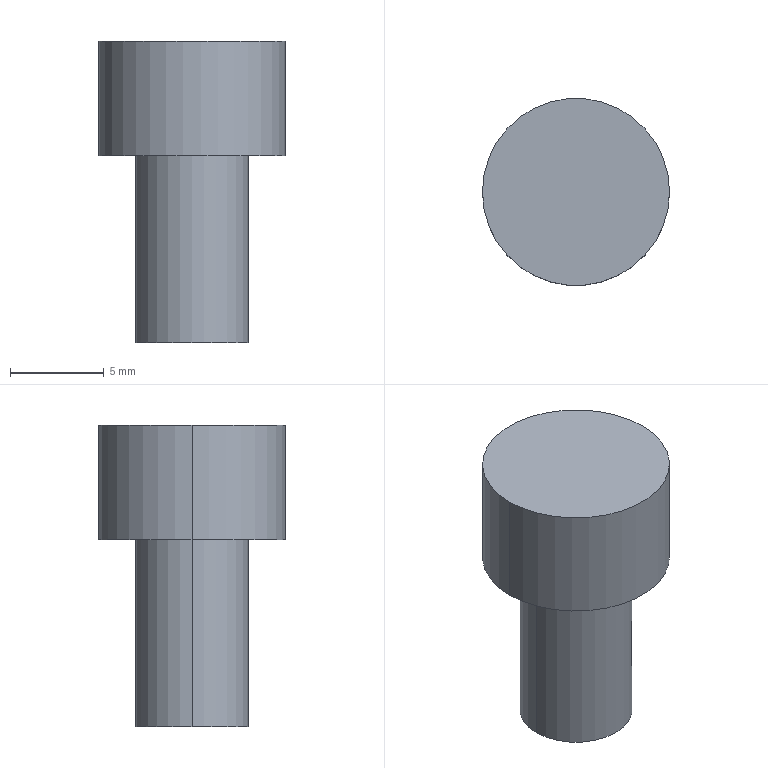Part | STEP file | m6-15 | 1 solid | 7 faces | box 10 x 10 x 16.1 mm | volume 761.836 mm3 | cylinder 4 | plane 3 | commonest cylinder face diameters 6 x2 10 x2
STEP:
#1=CARTESIAN_POINT('',(0.,0.,0.));
#2=DIRECTION('',(0.,0.,1.));
#3=DIRECTION('',(1.,0.,0.));
#4=AXIS2_PLACEMENT_3D('',#1,#2,#3);
#5=CARTESIAN_POINT('',(-3.,0.,-10.));
#6=VERTEX_POINT('',#5);
#7=CARTESIAN_POINT('',(3.,0.,-10.));
#8=VERTEX_POINT('',#7);
#9=CARTESIAN_POINT('',(0.,0.,-10.));
#10=DIRECTION('',(0.,0.,-1.));
#11=DIRECTION('',(-1.,0.,0.));
#12=AXIS2_PLACEMENT_3D('',#9,#10,#11);
#13=CIRCLE('',#12,3.);
#14=CARTESIAN_POINT('',(0.,0.,-10.));
#15=DIRECTION('',(0.,0.,1.));
#16=DIRECTION('',(1.,0.,0.));
#17=AXIS2_PLACEMENT_3D('',#14,#15,#16);
#18=CYLINDRICAL_SURFACE('',#17,3.);
#19=CARTESIAN_POINT('',(3.142,0.));
#20=DIRECTION('',(-1.,0.));
#21=VECTOR('',#20,1.);
#22=LINE('',#19,#21);
#23=(GEOMETRIC_REPRESENTATION_CONTEXT(2)PARAMETRIC_REPRESENTATION_CONTEXT()REPRESENTATION_CONTEXT('',''));
#24=DEFINITIONAL_REPRESENTATION('',(#22),#23);
#25=PCURVE('',#18,#24);
#26=CARTESIAN_POINT('',(0.,0.,-10.));
#27=DIRECTION('',(0.,0.,-1.));
#28=DIRECTION('',(-1.,0.,0.));
#29=AXIS2_PLACEMENT_3D('',#26,#27,#28);
#30=PLANE('',#29);
#31=CARTESIAN_POINT('',(0.,0.));
#32=DIRECTION('',(1.,0.));
#33=AXIS2_PLACEMENT_2D('',#31,#32);
#34=CIRCLE('',#33,3.);
#35=(GEOMETRIC_REPRESENTATION_CONTEXT(2)PARAMETRIC_REPRESENTATION_CONTEXT()REPRESENTATION_CONTEXT('',''));
#36=DEFINITIONAL_REPRESENTATION('',(#34),#35);
#37=PCURVE('',#30,#36);
#38=SURFACE_CURVE('',#13,(#25,#37),.PCURVE_S1.);
#39=EDGE_CURVE('',#6,#8,#38,.T.);
#40=ORIENTED_EDGE('',*,*,#39,.F.);
#41=CARTESIAN_POINT('',(-3.,0.,0.));
#42=VERTEX_POINT('',#41);
#43=CARTESIAN_POINT('',(-3.,0.,-10.));
#44=DIRECTION('',(0.,0.,1.));
#45=VECTOR('',#44,1.);
#46=LINE('',#43,#45);
#47=CARTESIAN_POINT('',(3.142,0.));
#48=DIRECTION('',(0.,1.));
#49=VECTOR('',#48,1.);
#50=LINE('',#47,#49);
#51=(GEOMETRIC_REPRESENTATION_CONTEXT(2)PARAMETRIC_REPRESENTATION_CONTEXT()REPRESENTATION_CONTEXT('',''));
#52=DEFINITIONAL_REPRESENTATION('',(#50),#51);
#53=PCURVE('',#18,#52);
#54=CARTESIAN_POINT('',(0.,0.,-10.));
#55=DIRECTION('',(0.,0.,1.));
#56=DIRECTION('',(1.,0.,0.));
#57=AXIS2_PLACEMENT_3D('',#54,#55,#56);
#58=CYLINDRICAL_SURFACE('',#57,3.);
#59=CARTESIAN_POINT('',(3.142,0.));
#60=DIRECTION('',(0.,1.));
#61=VECTOR('',#60,1.);
#62=LINE('',#59,#61);
#63=(GEOMETRIC_REPRESENTATION_CONTEXT(2)PARAMETRIC_REPRESENTATION_CONTEXT()REPRESENTATION_CONTEXT('',''));
#64=DEFINITIONAL_REPRESENTATION('',(#62),#63);
#65=PCURVE('',#58,#64);
#66=SURFACE_CURVE('',#46,(#53,#65),.PCURVE_S1.);
#67=EDGE_CURVE('',#6,#42,#66,.T.);
#68=ORIENTED_EDGE('',*,*,#67,.T.);
#69=CARTESIAN_POINT('',(3.,0.,0.));
#70=VERTEX_POINT('',#69);
#71=CARTESIAN_POINT('',(0.,0.,0.));
#72=DIRECTION('',(0.,0.,-1.));
#73=DIRECTION('',(1.,0.,0.));
#74=AXIS2_PLACEMENT_3D('',#71,#72,#73);
#75=CIRCLE('',#74,3.);
#76=CARTESIAN_POINT('',(6.283,10.));
#77=DIRECTION('',(-1.,0.));
#78=VECTOR('',#77,1.);
#79=LINE('',#76,#78);
#80=(GEOMETRIC_REPRESENTATION_CONTEXT(2)PARAMETRIC_REPRESENTATION_CONTEXT()REPRESENTATION_CONTEXT('',''));
#81=DEFINITIONAL_REPRESENTATION('',(#79),#80);
#82=PCURVE('',#18,#81);
#83=CARTESIAN_POINT('',(0.,0.,0.));
#84=DIRECTION('',(0.,0.,1.));
#85=DIRECTION('',(1.,0.,0.));
#86=AXIS2_PLACEMENT_3D('',#83,#84,#85);
#87=PLANE('',#86);
#88=CARTESIAN_POINT('',(3.,0.));
#89=CARTESIAN_POINT('',(3.,-5.196));
#90=CARTESIAN_POINT('',(-1.5,-2.598));
#91=CARTESIAN_POINT('',(-6.,0.));
#92=CARTESIAN_POINT('',(-1.5,2.598));
#93=CARTESIAN_POINT('',(3.,5.196));
#94=CARTESIAN_POINT('',(3.,0.));
#95=(BOUNDED_CURVE()B_SPLINE_CURVE(2,(#88,#89,#90,#91,#92,#93,#94),.UNSPECIFIED.,.T.,.F.)B_SPLINE_CURVE_WITH_KNOTS((1,2,2,2,2,1),(-2.094,0.,2.094,4.189,6.283,8.378),.UNSPECIFIED.)CURVE()GEOMETRIC_REPRESENTATION_ITEM()RATIONAL_B_SPLINE_CURVE((1.,0.5,1.,0.5,1.,0.5,1.))REPRESENTATION_ITEM(''));
#96=(GEOMETRIC_REPRESENTATION_CONTEXT(2)PARAMETRIC_REPRESENTATION_CONTEXT()REPRESENTATION_CONTEXT('',''));
#97=DEFINITIONAL_REPRESENTATION('',(#95),#96);
#98=PCURVE('',#87,#97);
#99=SURFACE_CURVE('',#75,(#82,#98),.PCURVE_S1.);
#100=EDGE_CURVE('',#42,#70,#99,.T.);
#101=ORIENTED_EDGE('',*,*,#100,.T.);
#102=CARTESIAN_POINT('',(3.,0.,-10.));
#103=DIRECTION('',(0.,0.,1.));
#104=VECTOR('',#103,1.);
#105=LINE('',#102,#104);
#106=CARTESIAN_POINT('',(0.,0.));
#107=DIRECTION('',(0.,1.));
#108=VECTOR('',#107,1.);
#109=LINE('',#106,#108);
#110=(GEOMETRIC_REPRESENTATION_CONTEXT(2)PARAMETRIC_REPRESENTATION_CONTEXT()REPRESENTATION_CONTEXT('',''));
#111=DEFINITIONAL_REPRESENTATION('',(#109),#110);
#112=PCURVE('',#18,#111);
#113=CARTESIAN_POINT('',(6.283,0.));
#114=DIRECTION('',(0.,1.));
#115=VECTOR('',#114,1.);
#116=LINE('',#113,#115);
#117=(GEOMETRIC_REPRESENTATION_CONTEXT(2)PARAMETRIC_REPRESENTATION_CONTEXT()REPRESENTATION_CONTEXT('',''));
#118=DEFINITIONAL_REPRESENTATION('',(#116),#117);
#119=PCURVE('',#58,#118);
#120=SURFACE_CURVE('',#105,(#112,#119),.PCURVE_S1.);
#121=EDGE_CURVE('',#8,#70,#120,.T.);
#122=ORIENTED_EDGE('',*,*,#121,.F.);
#123=EDGE_LOOP('',(#40,#68,#101,#122));
#124=FACE_BOUND('',#123,.T.);
#125=ADVANCED_FACE('',(#124),#18,.T.);
#126=CARTESIAN_POINT('',(5.,0.,6.1));
#127=VERTEX_POINT('',#126);
#128=CARTESIAN_POINT('',(-5.,0.,6.1));
#129=VERTEX_POINT('',#128);
#130=CARTESIAN_POINT('',(0.,0.,6.1));
#131=DIRECTION('',(0.,0.,1.));
#132=DIRECTION('',(1.,0.,0.));
#133=AXIS2_PLACEMENT_3D('',#130,#131,#132);
#134=CIRCLE('',#133,5.);
#135=CARTESIAN_POINT('',(0.,0.,6.1));
#136=DIRECTION('',(0.,0.,-1.));
#137=DIRECTION('',(-1.,0.,0.));
#138=AXIS2_PLACEMENT_3D('',#135,#136,#137);
#139=CYLINDRICAL_SURFACE('',#138,5.);
#140=CARTESIAN_POINT('',(3.142,0.));
#141=DIRECTION('',(-1.,0.));
#142=VECTOR('',#141,1.);
#143=LINE('',#140,#142);
#144=(GEOMETRIC_REPRESENTATION_CONTEXT(2)PARAMETRIC_REPRESENTATION_CONTEXT()REPRESENTATION_CONTEXT('',''));
#145=DEFINITIONAL_REPRESENTATION('',(#143),#144);
#146=PCURVE('',#139,#145);
#147=CARTESIAN_POINT('',(0.,0.,6.1));
#148=DIRECTION('',(0.,0.,1.));
#149=DIRECTION('',(1.,0.,0.));
#150=AXIS2_PLACEMENT_3D('',#147,#148,#149);
#151=PLANE('',#150);
#152=CARTESIAN_POINT('',(0.,0.));
#153=DIRECTION('',(1.,0.));
#154=AXIS2_PLACEMENT_2D('',#152,#153);
#155=CIRCLE('',#154,5.);
#156=(GEOMETRIC_REPRESENTATION_CONTEXT(2)PARAMETRIC_REPRESENTATION_CONTEXT()REPRESENTATION_CONTEXT('',''));
#157=DEFINITIONAL_REPRESENTATION('',(#155),#156);
#158=PCURVE('',#151,#157);
#159=SURFACE_CURVE('',#134,(#146,#158),.PCURVE_S1.);
#160=EDGE_CURVE('',#127,#129,#159,.T.);
#161=ORIENTED_EDGE('',*,*,#160,.F.);
#162=CARTESIAN_POINT('',(5.,0.,0.));
#163=VERTEX_POINT('',#162);
#164=CARTESIAN_POINT('',(5.,0.,6.1));
#165=DIRECTION('',(0.,0.,-1.));
#166=VECTOR('',#165,1.);
#167=LINE('',#164,#166);
#168=CARTESIAN_POINT('',(3.142,0.));
#169=DIRECTION('',(0.,1.));
#170=VECTOR('',#169,1.);
#171=LINE('',#168,#170);
#172=(GEOMETRIC_REPRESENTATION_CONTEXT(2)PARAMETRIC_REPRESENTATION_CONTEXT()REPRESENTATION_CONTEXT('',''));
#173=DEFINITIONAL_REPRESENTATION('',(#171),#172);
#174=PCURVE('',#139,#173);
#175=CARTESIAN_POINT('',(0.,0.,6.1));
#176=DIRECTION('',(0.,0.,-1.));
#177=DIRECTION('',(-1.,0.,0.));
#178=AXIS2_PLACEMENT_3D('',#175,#176,#177);
#179=CYLINDRICAL_SURFACE('',#178,5.);
#180=CARTESIAN_POINT('',(3.142,0.));
#181=DIRECTION('',(0.,1.));
#182=VECTOR('',#181,1.);
#183=LINE('',#180,#182);
#184=(GEOMETRIC_REPRESENTATION_CONTEXT(2)PARAMETRIC_REPRESENTATION_CONTEXT()REPRESENTATION_CONTEXT('',''));
#185=DEFINITIONAL_REPRESENTATION('',(#183),#184);
#186=PCURVE('',#179,#185);
#187=SURFACE_CURVE('',#167,(#174,#186),.PCURVE_S1.);
#188=EDGE_CURVE('',#127,#163,#187,.T.);
#189=ORIENTED_EDGE('',*,*,#188,.T.);
#190=CARTESIAN_POINT('',(-5.,0.,0.));
#191=VERTEX_POINT('',#190);
#192=CARTESIAN_POINT('',(0.,0.,0.));
#193=DIRECTION('',(0.,0.,1.));
#194=DIRECTION('',(1.,0.,0.));
#195=AXIS2_PLACEMENT_3D('',#192,#193,#194);
#196=CIRCLE('',#195,5.);
#197=CARTESIAN_POINT('',(3.142,6.1));
#198=DIRECTION('',(-1.,0.));
#199=VECTOR('',#198,1.);
#200=LINE('',#197,#199);
#201=(GEOMETRIC_REPRESENTATION_CONTEXT(2)PARAMETRIC_REPRESENTATION_CONTEXT()REPRESENTATION_CONTEXT('',''));
#202=DEFINITIONAL_REPRESENTATION('',(#200),#201);
#203=PCURVE('',#139,#202);
#204=CARTESIAN_POINT('',(0.,0.));
#205=DIRECTION('',(1.,0.));
#206=AXIS2_PLACEMENT_2D('',#204,#205);
#207=CIRCLE('',#206,5.);
#208=(GEOMETRIC_REPRESENTATION_CONTEXT(2)PARAMETRIC_REPRESENTATION_CONTEXT()REPRESENTATION_CONTEXT('',''));
#209=DEFINITIONAL_REPRESENTATION('',(#207),#208);
#210=PCURVE('',#87,#209);
#211=SURFACE_CURVE('',#196,(#203,#210),.PCURVE_S1.);
#212=EDGE_CURVE('',#163,#191,#211,.T.);
#213=ORIENTED_EDGE('',*,*,#212,.T.);
#214=CARTESIAN_POINT('',(-5.,0.,6.1));
#215=DIRECTION('',(0.,0.,-1.));
#216=VECTOR('',#215,1.);
#217=LINE('',#214,#216);
#218=CARTESIAN_POINT('',(0.,0.));
#219=DIRECTION('',(0.,1.));
#220=VECTOR('',#219,1.);
#221=LINE('',#218,#220);
#222=(GEOMETRIC_REPRESENTATION_CONTEXT(2)PARAMETRIC_REPRESENTATION_CONTEXT()REPRESENTATION_CONTEXT('',''));
#223=DEFINITIONAL_REPRESENTATION('',(#221),#222);
#224=PCURVE('',#139,#223);
#225=CARTESIAN_POINT('',(6.283,0.));
#226=DIRECTION('',(0.,1.));
#227=VECTOR('',#226,1.);
#228=LINE('',#225,#227);
#229=(GEOMETRIC_REPRESENTATION_CONTEXT(2)PARAMETRIC_REPRESENTATION_CONTEXT()REPRESENTATION_CONTEXT('',''));
#230=DEFINITIONAL_REPRESENTATION('',(#228),#229);
#231=PCURVE('',#179,#230);
#232=SURFACE_CURVE('',#217,(#224,#231),.PCURVE_S1.);
#233=EDGE_CURVE('',#129,#191,#232,.T.);
#234=ORIENTED_EDGE('',*,*,#233,.F.);
#235=EDGE_LOOP('',(#161,#189,#213,#234));
#236=FACE_BOUND('',#235,.T.);
#237=ADVANCED_FACE('',(#236),#139,.T.);
#238=CARTESIAN_POINT('',(0.,0.,0.));
#239=DIRECTION('',(0.,0.,1.));
#240=DIRECTION('',(1.,0.,0.));
#241=AXIS2_PLACEMENT_3D('',#238,#239,#240);
#242=CIRCLE('',#241,5.);
#243=CARTESIAN_POINT('',(0.,0.));
#244=DIRECTION('',(1.,0.));
#245=AXIS2_PLACEMENT_2D('',#243,#244);
#246=CIRCLE('',#245,5.);
#247=(GEOMETRIC_REPRESENTATION_CONTEXT(2)PARAMETRIC_REPRESENTATION_CONTEXT()REPRESENTATION_CONTEXT('',''));
#248=DEFINITIONAL_REPRESENTATION('',(#246),#247);
#249=PCURVE('',#87,#248);
#250=CARTESIAN_POINT('',(9.425,6.1));
#251=DIRECTION('',(-1.,0.));
#252=VECTOR('',#251,1.);
#253=LINE('',#250,#252);
#254=(GEOMETRIC_REPRESENTATION_CONTEXT(2)PARAMETRIC_REPRESENTATION_CONTEXT()REPRESENTATION_CONTEXT('',''));
#255=DEFINITIONAL_REPRESENTATION('',(#253),#254);
#256=PCURVE('',#179,#255);
#257=SURFACE_CURVE('',#242,(#249,#256),.PCURVE_S1.);
#258=EDGE_CURVE('',#191,#163,#257,.T.);
#259=ORIENTED_EDGE('',*,*,#258,.F.);
#260=ORIENTED_EDGE('',*,*,#212,.F.);
#261=EDGE_LOOP('',(#259,#260));
#262=FACE_BOUND('',#261,.T.);
#263=CARTESIAN_POINT('',(0.,0.,0.));
#264=DIRECTION('',(0.,0.,-1.));
#265=DIRECTION('',(1.,0.,0.));
#266=AXIS2_PLACEMENT_3D('',#263,#264,#265);
#267=CIRCLE('',#266,3.);
#268=CARTESIAN_POINT('',(3.,0.));
#269=CARTESIAN_POINT('',(3.,-5.196));
#270=CARTESIAN_POINT('',(-1.5,-2.598));
#271=CARTESIAN_POINT('',(-6.,0.));
#272=CARTESIAN_POINT('',(-1.5,2.598));
#273=CARTESIAN_POINT('',(3.,5.196));
#274=CARTESIAN_POINT('',(3.,0.));
#275=(BOUNDED_CURVE()B_SPLINE_CURVE(2,(#268,#269,#270,#271,#272,#273,#274),.UNSPECIFIED.,.T.,.F.)B_SPLINE_CURVE_WITH_KNOTS((1,2,2,2,2,1),(-2.094,0.,2.094,4.189,6.283,8.378),.UNSPECIFIED.)CURVE()GEOMETRIC_REPRESENTATION_ITEM()RATIONAL_B_SPLINE_CURVE((1.,0.5,1.,0.5,1.,0.5,1.))REPRESENTATION_ITEM(''));
#276=(GEOMETRIC_REPRESENTATION_CONTEXT(2)PARAMETRIC_REPRESENTATION_CONTEXT()REPRESENTATION_CONTEXT('',''));
#277=DEFINITIONAL_REPRESENTATION('',(#275),#276);
#278=PCURVE('',#87,#277);
#279=CARTESIAN_POINT('',(6.283,10.));
#280=DIRECTION('',(-1.,0.));
#281=VECTOR('',#280,1.);
#282=LINE('',#279,#281);
#283=(GEOMETRIC_REPRESENTATION_CONTEXT(2)PARAMETRIC_REPRESENTATION_CONTEXT()REPRESENTATION_CONTEXT('',''));
#284=DEFINITIONAL_REPRESENTATION('',(#282),#283);
#285=PCURVE('',#58,#284);
#286=SURFACE_CURVE('',#267,(#278,#285),.PCURVE_S1.);
#287=EDGE_CURVE('',#70,#42,#286,.T.);
#288=ORIENTED_EDGE('',*,*,#287,.F.);
#289=ORIENTED_EDGE('',*,*,#100,.F.);
#290=EDGE_LOOP('',(#288,#289));
#291=FACE_BOUND('',#290,.T.);
#292=ADVANCED_FACE('',(#262,#291),#87,.F.);
#293=ORIENTED_EDGE('',*,*,#188,.F.);
#294=CARTESIAN_POINT('',(0.,0.,6.1));
#295=DIRECTION('',(0.,0.,1.));
#296=DIRECTION('',(1.,0.,0.));
#297=AXIS2_PLACEMENT_3D('',#294,#295,#296);
#298=CIRCLE('',#297,5.);
#299=CARTESIAN_POINT('',(9.425,0.));
#300=DIRECTION('',(-1.,0.));
#301=VECTOR('',#300,1.);
#302=LINE('',#299,#301);
#303=(GEOMETRIC_REPRESENTATION_CONTEXT(2)PARAMETRIC_REPRESENTATION_CONTEXT()REPRESENTATION_CONTEXT('',''));
#304=DEFINITIONAL_REPRESENTATION('',(#302),#303);
#305=PCURVE('',#179,#304);
#306=CARTESIAN_POINT('',(0.,0.));
#307=DIRECTION('',(1.,0.));
#308=AXIS2_PLACEMENT_2D('',#306,#307);
#309=CIRCLE('',#308,5.);
#310=(GEOMETRIC_REPRESENTATION_CONTEXT(2)PARAMETRIC_REPRESENTATION_CONTEXT()REPRESENTATION_CONTEXT('',''));
#311=DEFINITIONAL_REPRESENTATION('',(#309),#310);
#312=PCURVE('',#151,#311);
#313=SURFACE_CURVE('',#298,(#305,#312),.PCURVE_S1.);
#314=EDGE_CURVE('',#129,#127,#313,.T.);
#315=ORIENTED_EDGE('',*,*,#314,.F.);
#316=ORIENTED_EDGE('',*,*,#233,.T.);
#317=ORIENTED_EDGE('',*,*,#258,.T.);
#318=EDGE_LOOP('',(#293,#315,#316,#317));
#319=FACE_BOUND('',#318,.T.);
#320=ADVANCED_FACE('',(#319),#179,.T.);
#321=ORIENTED_EDGE('',*,*,#314,.T.);
#322=ORIENTED_EDGE('',*,*,#160,.T.);
#323=EDGE_LOOP('',(#321,#322));
#324=FACE_BOUND('',#323,.T.);
#325=ADVANCED_FACE('',(#324),#151,.T.);
#326=ORIENTED_EDGE('',*,*,#67,.F.);
#327=CARTESIAN_POINT('',(0.,0.,-10.));
#328=DIRECTION('',(0.,0.,-1.));
#329=DIRECTION('',(-1.,0.,0.));
#330=AXIS2_PLACEMENT_3D('',#327,#328,#329);
#331=CIRCLE('',#330,3.);
#332=CARTESIAN_POINT('',(9.425,0.));
#333=DIRECTION('',(-1.,0.));
#334=VECTOR('',#333,1.);
#335=LINE('',#332,#334);
#336=(GEOMETRIC_REPRESENTATION_CONTEXT(2)PARAMETRIC_REPRESENTATION_CONTEXT()REPRESENTATION_CONTEXT('',''));
#337=DEFINITIONAL_REPRESENTATION('',(#335),#336);
#338=PCURVE('',#58,#337);
#339=CARTESIAN_POINT('',(0.,0.));
#340=DIRECTION('',(1.,0.));
#341=AXIS2_PLACEMENT_2D('',#339,#340);
#342=CIRCLE('',#341,3.);
#343=(GEOMETRIC_REPRESENTATION_CONTEXT(2)PARAMETRIC_REPRESENTATION_CONTEXT()REPRESENTATION_CONTEXT('',''));
#344=DEFINITIONAL_REPRESENTATION('',(#342),#343);
#345=PCURVE('',#30,#344);
#346=SURFACE_CURVE('',#331,(#338,#345),.PCURVE_S1.);
#347=EDGE_CURVE('',#8,#6,#346,.T.);
#348=ORIENTED_EDGE('',*,*,#347,.F.);
#349=ORIENTED_EDGE('',*,*,#121,.T.);
#350=ORIENTED_EDGE('',*,*,#287,.T.);
#351=EDGE_LOOP('',(#326,#348,#349,#350));
#352=FACE_BOUND('',#351,.T.);
#353=ADVANCED_FACE('',(#352),#58,.T.);
#354=ORIENTED_EDGE('',*,*,#347,.T.);
#355=ORIENTED_EDGE('',*,*,#39,.T.);
#356=EDGE_LOOP('',(#354,#355));
#357=FACE_BOUND('',#356,.T.);
#358=ADVANCED_FACE('',(#357),#30,.T.);
#359=CLOSED_SHELL('',(#125,#237,#292,#320,#325,#353,#358));
#360=MANIFOLD_SOLID_BREP('',#359);
#361=(LENGTH_UNIT()NAMED_UNIT(*)SI_UNIT(.MILLI.,.METRE.));
#362=UNCERTAINTY_MEASURE_WITH_UNIT(LENGTH_MEASURE(0.0000001),#361,'','');
#363=(NAMED_UNIT(*)PLANE_ANGLE_UNIT()SI_UNIT($,.RADIAN.));
#364=(NAMED_UNIT(*)SI_UNIT($,.STERADIAN.)SOLID_ANGLE_UNIT());
#365=(GEOMETRIC_REPRESENTATION_CONTEXT(3)GLOBAL_UNCERTAINTY_ASSIGNED_CONTEXT((#362))GLOBAL_UNIT_ASSIGNED_CONTEXT((#361,#363,#364))REPRESENTATION_CONTEXT('',''));
#366=ADVANCED_BREP_SHAPE_REPRESENTATION('',(#4,#360),#365);